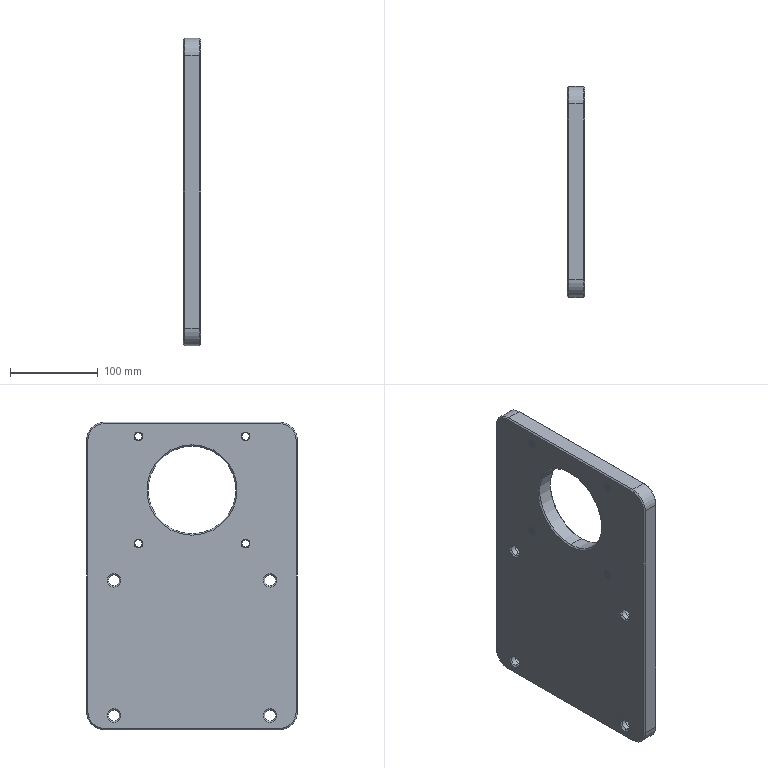Part | SolidWorks | features BaseBody 1 | 1 solid | 202 faces | box 20 x 240 x 350 mm | volume 1488667 mm3 | cylinder 126 | cone 50 | plane 18 | spline 8 | commonest cylinder face diameters 8.5 x104 12.5 x8 19 x8 40 x4 100 x2